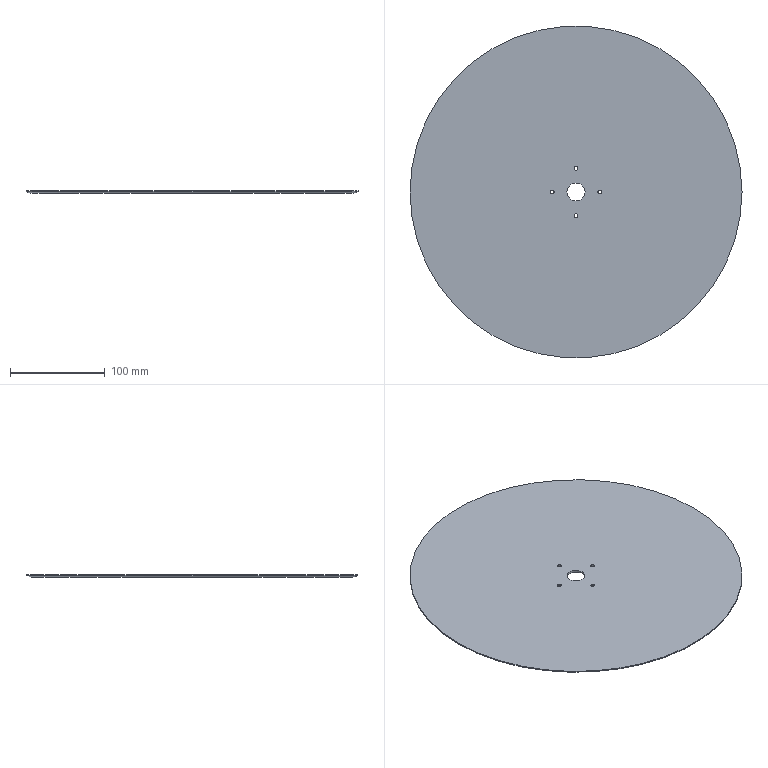Part | SolidWorks | features ICE 3, Extrusion 1, Sweep 1 | 1 solid | 16 faces | box 350 x 350 x 2.3 mm | volume 217251 mm3 | cylinder 12 | cone 2 | plane 2 | commonest cylinder face diameters 4 x8 19 x2 350 x2
STEP:
#1=CARTESIAN_POINT('',(-27.,0.,-1.2));
#2=VERTEX_POINT('',#1);
#3=CARTESIAN_POINT('',(-23.,0.,-1.2));
#4=VERTEX_POINT('',#3);
#5=CARTESIAN_POINT('',(-25.,0.,-1.2));
#6=DIRECTION('',(0.,0.,1.));
#7=DIRECTION('',(-1.,0.,0.));
#8=AXIS2_PLACEMENT_3D('',#5,#6,#7);
#9=CIRCLE('',#8,2.);
#10=EDGE_CURVE('',#2,#4,#9,.T.);
#11=ORIENTED_EDGE('',*,*,#10,.F.);
#12=CARTESIAN_POINT('',(-27.,0.,1.1));
#13=VERTEX_POINT('',#12);
#14=CARTESIAN_POINT('',(-27.,0.,-6.857));
#15=DIRECTION('',(0.,0.,1.));
#16=VECTOR('',#15,1000.);
#17=LINE('',#14,#16);
#18=EDGE_CURVE('',#2,#13,#17,.T.);
#19=ORIENTED_EDGE('',*,*,#18,.T.);
#20=CARTESIAN_POINT('',(-23.,0.,1.1));
#21=VERTEX_POINT('',#20);
#22=CARTESIAN_POINT('',(-25.,0.,1.1));
#23=DIRECTION('',(0.,0.,1.));
#24=DIRECTION('',(1.,0.,0.));
#25=AXIS2_PLACEMENT_3D('',#22,#23,#24);
#26=CIRCLE('',#25,2.);
#27=EDGE_CURVE('',#13,#21,#26,.T.);
#28=ORIENTED_EDGE('',*,*,#27,.T.);
#29=CARTESIAN_POINT('',(-23.,0.,-6.857));
#30=DIRECTION('',(0.,0.,1.));
#31=VECTOR('',#30,1000.);
#32=LINE('',#29,#31);
#33=EDGE_CURVE('',#4,#21,#32,.T.);
#34=ORIENTED_EDGE('',*,*,#33,.F.);
#35=EDGE_LOOP('',(#11,#19,#28,#34));
#36=FACE_OUTER_BOUND('',#35,.T.);
#37=CARTESIAN_POINT('',(-25.,0.,-6.857));
#38=DIRECTION('',(0.,0.,1.));
#39=DIRECTION('',(1.,0.,0.));
#40=AXIS2_PLACEMENT_3D('',#37,#38,#39);
#41=CYLINDRICAL_SURFACE('',#40,2.);
#42=ADVANCED_FACE('',(#36),#41,.F.);
#43=CARTESIAN_POINT('',(-2.,-25.,-1.2));
#44=VERTEX_POINT('',#43);
#45=CARTESIAN_POINT('',(2.,-25.,-1.2));
#46=VERTEX_POINT('',#45);
#47=CARTESIAN_POINT('',(0.,-25.,-1.2));
#48=DIRECTION('',(0.,0.,1.));
#49=DIRECTION('',(-1.,0.,0.));
#50=AXIS2_PLACEMENT_3D('',#47,#48,#49);
#51=CIRCLE('',#50,2.);
#52=EDGE_CURVE('',#44,#46,#51,.T.);
#53=ORIENTED_EDGE('',*,*,#52,.F.);
#54=CARTESIAN_POINT('',(-2.,-25.,1.1));
#55=VERTEX_POINT('',#54);
#56=CARTESIAN_POINT('',(-2.,-25.,-6.857));
#57=DIRECTION('',(0.,0.,1.));
#58=VECTOR('',#57,1000.);
#59=LINE('',#56,#58);
#60=EDGE_CURVE('',#44,#55,#59,.T.);
#61=ORIENTED_EDGE('',*,*,#60,.T.);
#62=CARTESIAN_POINT('',(2.,-25.,1.1));
#63=VERTEX_POINT('',#62);
#64=CARTESIAN_POINT('',(0.,-25.,1.1));
#65=DIRECTION('',(0.,0.,1.));
#66=DIRECTION('',(1.,0.,0.));
#67=AXIS2_PLACEMENT_3D('',#64,#65,#66);
#68=CIRCLE('',#67,2.);
#69=EDGE_CURVE('',#55,#63,#68,.T.);
#70=ORIENTED_EDGE('',*,*,#69,.T.);
#71=CARTESIAN_POINT('',(2.,-25.,-6.857));
#72=DIRECTION('',(0.,0.,1.));
#73=VECTOR('',#72,1000.);
#74=LINE('',#71,#73);
#75=EDGE_CURVE('',#46,#63,#74,.T.);
#76=ORIENTED_EDGE('',*,*,#75,.F.);
#77=EDGE_LOOP('',(#53,#61,#70,#76));
#78=FACE_OUTER_BOUND('',#77,.T.);
#79=CARTESIAN_POINT('',(0.,-25.,-6.857));
#80=DIRECTION('',(0.,0.,1.));
#81=DIRECTION('',(1.,0.,0.));
#82=AXIS2_PLACEMENT_3D('',#79,#80,#81);
#83=CYLINDRICAL_SURFACE('',#82,2.);
#84=ADVANCED_FACE('',(#78),#83,.F.);
#85=CARTESIAN_POINT('',(23.,0.,-1.2));
#86=VERTEX_POINT('',#85);
#87=CARTESIAN_POINT('',(27.,0.,-1.2));
#88=VERTEX_POINT('',#87);
#89=CARTESIAN_POINT('',(25.,0.,-1.2));
#90=DIRECTION('',(0.,0.,1.));
#91=DIRECTION('',(-1.,0.,0.));
#92=AXIS2_PLACEMENT_3D('',#89,#90,#91);
#93=CIRCLE('',#92,2.);
#94=EDGE_CURVE('',#86,#88,#93,.T.);
#95=ORIENTED_EDGE('',*,*,#94,.F.);
#96=CARTESIAN_POINT('',(23.,0.,1.1));
#97=VERTEX_POINT('',#96);
#98=CARTESIAN_POINT('',(23.,0.,-6.857));
#99=DIRECTION('',(0.,0.,1.));
#100=VECTOR('',#99,1000.);
#101=LINE('',#98,#100);
#102=EDGE_CURVE('',#86,#97,#101,.T.);
#103=ORIENTED_EDGE('',*,*,#102,.T.);
#104=CARTESIAN_POINT('',(27.,0.,1.1));
#105=VERTEX_POINT('',#104);
#106=CARTESIAN_POINT('',(25.,0.,1.1));
#107=DIRECTION('',(0.,0.,1.));
#108=DIRECTION('',(1.,0.,0.));
#109=AXIS2_PLACEMENT_3D('',#106,#107,#108);
#110=CIRCLE('',#109,2.);
#111=EDGE_CURVE('',#97,#105,#110,.T.);
#112=ORIENTED_EDGE('',*,*,#111,.T.);
#113=CARTESIAN_POINT('',(27.,0.,-6.857));
#114=DIRECTION('',(0.,0.,1.));
#115=VECTOR('',#114,1000.);
#116=LINE('',#113,#115);
#117=EDGE_CURVE('',#88,#105,#116,.T.);
#118=ORIENTED_EDGE('',*,*,#117,.F.);
#119=EDGE_LOOP('',(#95,#103,#112,#118));
#120=FACE_OUTER_BOUND('',#119,.T.);
#121=CARTESIAN_POINT('',(25.,0.,-6.857));
#122=DIRECTION('',(0.,0.,1.));
#123=DIRECTION('',(1.,0.,0.));
#124=AXIS2_PLACEMENT_3D('',#121,#122,#123);
#125=CYLINDRICAL_SURFACE('',#124,2.);
#126=ADVANCED_FACE('',(#120),#125,.F.);
#127=CARTESIAN_POINT('',(-2.,25.,-1.2));
#128=VERTEX_POINT('',#127);
#129=CARTESIAN_POINT('',(2.,25.,-1.2));
#130=VERTEX_POINT('',#129);
#131=CARTESIAN_POINT('',(0.,25.,-1.2));
#132=DIRECTION('',(0.,0.,1.));
#133=DIRECTION('',(-1.,0.,0.));
#134=AXIS2_PLACEMENT_3D('',#131,#132,#133);
#135=CIRCLE('',#134,2.);
#136=EDGE_CURVE('',#128,#130,#135,.T.);
#137=ORIENTED_EDGE('',*,*,#136,.F.);
#138=CARTESIAN_POINT('',(-2.,25.,1.1));
#139=VERTEX_POINT('',#138);
#140=CARTESIAN_POINT('',(-2.,25.,-6.857));
#141=DIRECTION('',(0.,0.,1.));
#142=VECTOR('',#141,1000.);
#143=LINE('',#140,#142);
#144=EDGE_CURVE('',#128,#139,#143,.T.);
#145=ORIENTED_EDGE('',*,*,#144,.T.);
#146=CARTESIAN_POINT('',(2.,25.,1.1));
#147=VERTEX_POINT('',#146);
#148=CARTESIAN_POINT('',(0.,25.,1.1));
#149=DIRECTION('',(0.,0.,1.));
#150=DIRECTION('',(1.,0.,0.));
#151=AXIS2_PLACEMENT_3D('',#148,#149,#150);
#152=CIRCLE('',#151,2.);
#153=EDGE_CURVE('',#139,#147,#152,.T.);
#154=ORIENTED_EDGE('',*,*,#153,.T.);
#155=CARTESIAN_POINT('',(2.,25.,-6.857));
#156=DIRECTION('',(0.,0.,1.));
#157=VECTOR('',#156,1000.);
#158=LINE('',#155,#157);
#159=EDGE_CURVE('',#130,#147,#158,.T.);
#160=ORIENTED_EDGE('',*,*,#159,.F.);
#161=EDGE_LOOP('',(#137,#145,#154,#160));
#162=FACE_OUTER_BOUND('',#161,.T.);
#163=CARTESIAN_POINT('',(0.,25.,-6.857));
#164=DIRECTION('',(0.,0.,1.));
#165=DIRECTION('',(1.,0.,0.));
#166=AXIS2_PLACEMENT_3D('',#163,#164,#165);
#167=CYLINDRICAL_SURFACE('',#166,2.);
#168=ADVANCED_FACE('',(#162),#167,.F.);
#169=CARTESIAN_POINT('',(170.,0.,-1.2));
#170=VERTEX_POINT('',#169);
#171=CARTESIAN_POINT('',(-170.,0.,-1.2));
#172=VERTEX_POINT('',#171);
#173=CARTESIAN_POINT('',(0.,0.,-1.2));
#174=DIRECTION('',(0.,0.,1.));
#175=DIRECTION('',(1.,0.,0.));
#176=AXIS2_PLACEMENT_3D('',#173,#174,#175);
#177=CIRCLE('',#176,170.);
#178=EDGE_CURVE('',#170,#172,#177,.T.);
#179=ORIENTED_EDGE('',*,*,#178,.T.);
#180=CARTESIAN_POINT('',(-175.,0.,0.));
#181=VERTEX_POINT('',#180);
#182=CARTESIAN_POINT('',(-170.,0.,-1.2));
#183=DIRECTION('',(-0.9724,0.,0.2334));
#184=VECTOR('',#183,1000.);
#185=LINE('',#182,#184);
#186=EDGE_CURVE('',#172,#181,#185,.T.);
#187=ORIENTED_EDGE('',*,*,#186,.T.);
#188=CARTESIAN_POINT('',(175.,0.,0.));
#189=VERTEX_POINT('',#188);
#190=CARTESIAN_POINT('',(0.,0.,0.));
#191=DIRECTION('',(0.,0.,1.));
#192=DIRECTION('',(1.,0.,0.));
#193=AXIS2_PLACEMENT_3D('',#190,#191,#192);
#194=CIRCLE('',#193,175.);
#195=EDGE_CURVE('',#189,#181,#194,.T.);
#196=ORIENTED_EDGE('',*,*,#195,.F.);
#197=CARTESIAN_POINT('',(170.,0.,-1.2));
#198=DIRECTION('',(0.9724,0.,0.2334));
#199=VECTOR('',#198,1000.);
#200=LINE('',#197,#199);
#201=EDGE_CURVE('',#170,#189,#200,.T.);
#202=ORIENTED_EDGE('',*,*,#201,.F.);
#203=EDGE_LOOP('',(#179,#187,#196,#202));
#204=FACE_OUTER_BOUND('',#203,.T.);
#205=CARTESIAN_POINT('',(0.,0.,-1.2));
#206=DIRECTION('',(0.,0.,1.));
#207=DIRECTION('',(1.,0.,0.));
#208=AXIS2_PLACEMENT_3D('',#205,#206,#207);
#209=CONICAL_SURFACE('',#208,170.,1.335);
#210=ADVANCED_FACE('',(#204),#209,.T.);
#211=CARTESIAN_POINT('',(-9.5,0.,-1.2));
#212=VERTEX_POINT('',#211);
#213=CARTESIAN_POINT('',(9.5,0.,-1.2));
#214=VERTEX_POINT('',#213);
#215=CARTESIAN_POINT('',(0.,0.,-1.2));
#216=DIRECTION('',(0.,0.,1.));
#217=DIRECTION('',(1.,0.,0.));
#218=AXIS2_PLACEMENT_3D('',#215,#216,#217);
#219=CIRCLE('',#218,9.5);
#220=EDGE_CURVE('',#212,#214,#219,.T.);
#221=ORIENTED_EDGE('',*,*,#220,.F.);
#222=CARTESIAN_POINT('',(-9.5,0.,1.1));
#223=VERTEX_POINT('',#222);
#224=CARTESIAN_POINT('',(-9.5,0.,-1.2));
#225=DIRECTION('',(0.,0.,1.));
#226=VECTOR('',#225,1000.);
#227=LINE('',#224,#226);
#228=EDGE_CURVE('',#212,#223,#227,.T.);
#229=ORIENTED_EDGE('',*,*,#228,.T.);
#230=CARTESIAN_POINT('',(9.5,0.,1.1));
#231=VERTEX_POINT('',#230);
#232=CARTESIAN_POINT('',(0.,0.,1.1));
#233=DIRECTION('',(0.,0.,1.));
#234=DIRECTION('',(1.,0.,0.));
#235=AXIS2_PLACEMENT_3D('',#232,#233,#234);
#236=CIRCLE('',#235,9.5);
#237=EDGE_CURVE('',#223,#231,#236,.T.);
#238=ORIENTED_EDGE('',*,*,#237,.T.);
#239=CARTESIAN_POINT('',(9.5,0.,-1.2));
#240=DIRECTION('',(0.,0.,1.));
#241=VECTOR('',#240,1000.);
#242=LINE('',#239,#241);
#243=EDGE_CURVE('',#214,#231,#242,.T.);
#244=ORIENTED_EDGE('',*,*,#243,.F.);
#245=EDGE_LOOP('',(#221,#229,#238,#244));
#246=FACE_OUTER_BOUND('',#245,.T.);
#247=CARTESIAN_POINT('',(0.,0.,-1.2));
#248=DIRECTION('',(0.,0.,1.));
#249=DIRECTION('',(1.,0.,0.));
#250=AXIS2_PLACEMENT_3D('',#247,#248,#249);
#251=CYLINDRICAL_SURFACE('',#250,9.5);
#252=ADVANCED_FACE('',(#246),#251,.F.);
#253=CARTESIAN_POINT('',(175.,0.,1.1));
#254=VERTEX_POINT('',#253);
#255=CARTESIAN_POINT('',(-175.,0.,1.1));
#256=VERTEX_POINT('',#255);
#257=CARTESIAN_POINT('',(0.,0.,1.1));
#258=DIRECTION('',(0.,0.,1.));
#259=DIRECTION('',(1.,0.,0.));
#260=AXIS2_PLACEMENT_3D('',#257,#258,#259);
#261=CIRCLE('',#260,175.);
#262=EDGE_CURVE('',#254,#256,#261,.T.);
#263=ORIENTED_EDGE('',*,*,#262,.F.);
#264=CARTESIAN_POINT('',(175.,0.,1.1));
#265=DIRECTION('',(0.,0.,-1.));
#266=VECTOR('',#265,1000.);
#267=LINE('',#264,#266);
#268=EDGE_CURVE('',#254,#189,#267,.T.);
#269=ORIENTED_EDGE('',*,*,#268,.T.);
#270=ORIENTED_EDGE('',*,*,#195,.T.);
#271=CARTESIAN_POINT('',(-175.,0.,1.1));
#272=DIRECTION('',(0.,0.,-1.));
#273=VECTOR('',#272,1000.);
#274=LINE('',#271,#273);
#275=EDGE_CURVE('',#256,#181,#274,.T.);
#276=ORIENTED_EDGE('',*,*,#275,.F.);
#277=EDGE_LOOP('',(#263,#269,#270,#276));
#278=FACE_OUTER_BOUND('',#277,.T.);
#279=CARTESIAN_POINT('',(0.,0.,1.1));
#280=DIRECTION('',(0.,0.,-1.));
#281=DIRECTION('',(-1.,0.,0.));
#282=AXIS2_PLACEMENT_3D('',#279,#280,#281);
#283=CYLINDRICAL_SURFACE('',#282,175.);
#284=ADVANCED_FACE('',(#278),#283,.T.);
#285=ORIENTED_EDGE('',*,*,#268,.F.);
#286=CARTESIAN_POINT('',(0.,0.,1.1));
#287=DIRECTION('',(0.,0.,1.));
#288=DIRECTION('',(1.,0.,0.));
#289=AXIS2_PLACEMENT_3D('',#286,#287,#288);
#290=CIRCLE('',#289,175.);
#291=EDGE_CURVE('',#256,#254,#290,.T.);
#292=ORIENTED_EDGE('',*,*,#291,.F.);
#293=ORIENTED_EDGE('',*,*,#275,.T.);
#294=CARTESIAN_POINT('',(0.,0.,0.));
#295=DIRECTION('',(0.,0.,1.));
#296=DIRECTION('',(1.,0.,0.));
#297=AXIS2_PLACEMENT_3D('',#294,#295,#296);
#298=CIRCLE('',#297,175.);
#299=EDGE_CURVE('',#181,#189,#298,.T.);
#300=ORIENTED_EDGE('',*,*,#299,.T.);
#301=EDGE_LOOP('',(#285,#292,#293,#300));
#302=FACE_OUTER_BOUND('',#301,.T.);
#303=CARTESIAN_POINT('',(0.,0.,1.1));
#304=DIRECTION('',(0.,0.,-1.));
#305=DIRECTION('',(-1.,0.,0.));
#306=AXIS2_PLACEMENT_3D('',#303,#304,#305);
#307=CYLINDRICAL_SURFACE('',#306,175.);
#308=ADVANCED_FACE('',(#302),#307,.T.);
#309=CARTESIAN_POINT('',(-25.,0.,1.1));
#310=DIRECTION('',(0.,0.,1.));
#311=DIRECTION('',(1.,0.,0.));
#312=AXIS2_PLACEMENT_3D('',#309,#310,#311);
#313=CIRCLE('',#312,2.);
#314=EDGE_CURVE('',#21,#13,#313,.T.);
#315=ORIENTED_EDGE('',*,*,#314,.F.);
#316=ORIENTED_EDGE('',*,*,#27,.F.);
#317=EDGE_LOOP('',(#315,#316));
#318=FACE_BOUND('',#317,.T.);
#319=CARTESIAN_POINT('',(0.,-25.,1.1));
#320=DIRECTION('',(0.,0.,1.));
#321=DIRECTION('',(1.,0.,0.));
#322=AXIS2_PLACEMENT_3D('',#319,#320,#321);
#323=CIRCLE('',#322,2.);
#324=EDGE_CURVE('',#63,#55,#323,.T.);
#325=ORIENTED_EDGE('',*,*,#324,.F.);
#326=ORIENTED_EDGE('',*,*,#69,.F.);
#327=EDGE_LOOP('',(#325,#326));
#328=FACE_BOUND('',#327,.T.);
#329=CARTESIAN_POINT('',(25.,0.,1.1));
#330=DIRECTION('',(0.,0.,1.));
#331=DIRECTION('',(1.,0.,0.));
#332=AXIS2_PLACEMENT_3D('',#329,#330,#331);
#333=CIRCLE('',#332,2.);
#334=EDGE_CURVE('',#105,#97,#333,.T.);
#335=ORIENTED_EDGE('',*,*,#334,.F.);
#336=ORIENTED_EDGE('',*,*,#111,.F.);
#337=EDGE_LOOP('',(#335,#336));
#338=FACE_BOUND('',#337,.T.);
#339=CARTESIAN_POINT('',(0.,25.,1.1));
#340=DIRECTION('',(0.,0.,1.));
#341=DIRECTION('',(1.,0.,0.));
#342=AXIS2_PLACEMENT_3D('',#339,#340,#341);
#343=CIRCLE('',#342,2.);
#344=EDGE_CURVE('',#147,#139,#343,.T.);
#345=ORIENTED_EDGE('',*,*,#344,.F.);
#346=ORIENTED_EDGE('',*,*,#153,.F.);
#347=EDGE_LOOP('',(#345,#346));
#348=FACE_BOUND('',#347,.T.);
#349=CARTESIAN_POINT('',(0.,0.,1.1));
#350=DIRECTION('',(0.,0.,1.));
#351=DIRECTION('',(1.,0.,0.));
#352=AXIS2_PLACEMENT_3D('',#349,#350,#351);
#353=CIRCLE('',#352,9.5);
#354=EDGE_CURVE('',#231,#223,#353,.T.);
#355=ORIENTED_EDGE('',*,*,#354,.F.);
#356=ORIENTED_EDGE('',*,*,#237,.F.);
#357=EDGE_LOOP('',(#355,#356));
#358=FACE_BOUND('',#357,.T.);
#359=ORIENTED_EDGE('',*,*,#291,.T.);
#360=ORIENTED_EDGE('',*,*,#262,.T.);
#361=EDGE_LOOP('',(#359,#360));
#362=FACE_OUTER_BOUND('',#361,.T.);
#363=CARTESIAN_POINT('',(0.,0.,1.1));
#364=DIRECTION('',(0.,0.,1.));
#365=DIRECTION('',(1.,0.,0.));
#366=AXIS2_PLACEMENT_3D('',#363,#364,#365);
#367=PLANE('',#366);
#368=ADVANCED_FACE('',(#318,#328,#338,#348,#358,#362),#367,.T.);
#369=CARTESIAN_POINT('',(-25.,0.,-1.2));
#370=DIRECTION('',(0.,0.,1.));
#371=DIRECTION('',(-1.,0.,0.));
#372=AXIS2_PLACEMENT_3D('',#369,#370,#371);
#373=CIRCLE('',#372,2.);
#374=EDGE_CURVE('',#4,#2,#373,.T.);
#375=ORIENTED_EDGE('',*,*,#374,.T.);
#376=ORIENTED_EDGE('',*,*,#10,.T.);
#377=EDGE_LOOP('',(#375,#376));
#378=FACE_BOUND('',#377,.T.);
#379=CARTESIAN_POINT('',(0.,-25.,-1.2));
#380=DIRECTION('',(0.,0.,1.));
#381=DIRECTION('',(-1.,0.,0.));
#382=AXIS2_PLACEMENT_3D('',#379,#380,#381);
#383=CIRCLE('',#382,2.);
#384=EDGE_CURVE('',#46,#44,#383,.T.);
#385=ORIENTED_EDGE('',*,*,#384,.T.);
#386=ORIENTED_EDGE('',*,*,#52,.T.);
#387=EDGE_LOOP('',(#385,#386));
#388=FACE_BOUND('',#387,.T.);
#389=CARTESIAN_POINT('',(25.,0.,-1.2));
#390=DIRECTION('',(0.,0.,1.));
#391=DIRECTION('',(-1.,0.,0.));
#392=AXIS2_PLACEMENT_3D('',#389,#390,#391);
#393=CIRCLE('',#392,2.);
#394=EDGE_CURVE('',#88,#86,#393,.T.);
#395=ORIENTED_EDGE('',*,*,#394,.T.);
#396=ORIENTED_EDGE('',*,*,#94,.T.);
#397=EDGE_LOOP('',(#395,#396));
#398=FACE_BOUND('',#397,.T.);
#399=CARTESIAN_POINT('',(0.,25.,-1.2));
#400=DIRECTION('',(0.,0.,1.));
#401=DIRECTION('',(-1.,0.,0.));
#402=AXIS2_PLACEMENT_3D('',#399,#400,#401);
#403=CIRCLE('',#402,2.);
#404=EDGE_CURVE('',#130,#128,#403,.T.);
#405=ORIENTED_EDGE('',*,*,#404,.T.);
#406=ORIENTED_EDGE('',*,*,#136,.T.);
#407=EDGE_LOOP('',(#405,#406));
#408=FACE_BOUND('',#407,.T.);
#409=CARTESIAN_POINT('',(0.,0.,-1.2));
#410=DIRECTION('',(0.,0.,1.));
#411=DIRECTION('',(1.,0.,0.));
#412=AXIS2_PLACEMENT_3D('',#409,#410,#411);
#413=CIRCLE('',#412,9.5);
#414=EDGE_CURVE('',#214,#212,#413,.T.);
#415=ORIENTED_EDGE('',*,*,#414,.T.);
#416=ORIENTED_EDGE('',*,*,#220,.T.);
#417=EDGE_LOOP('',(#415,#416));
#418=FACE_BOUND('',#417,.T.);
#419=ORIENTED_EDGE('',*,*,#178,.F.);
#420=CARTESIAN_POINT('',(0.,0.,-1.2));
#421=DIRECTION('',(0.,0.,1.));
#422=DIRECTION('',(1.,0.,0.));
#423=AXIS2_PLACEMENT_3D('',#420,#421,#422);
#424=CIRCLE('',#423,170.);
#425=EDGE_CURVE('',#172,#170,#424,.T.);
#426=ORIENTED_EDGE('',*,*,#425,.F.);
#427=EDGE_LOOP('',(#419,#426));
#428=FACE_OUTER_BOUND('',#427,.T.);
#429=CARTESIAN_POINT('',(0.,0.,-1.2));
#430=DIRECTION('',(0.,0.,-1.));
#431=DIRECTION('',(-1.,0.,0.));
#432=AXIS2_PLACEMENT_3D('',#429,#430,#431);
#433=PLANE('',#432);
#434=ADVANCED_FACE('',(#378,#388,#398,#408,#418,#428),#433,.T.);
#435=ORIENTED_EDGE('',*,*,#228,.F.);
#436=ORIENTED_EDGE('',*,*,#414,.F.);
#437=ORIENTED_EDGE('',*,*,#243,.T.);
#438=ORIENTED_EDGE('',*,*,#354,.T.);
#439=EDGE_LOOP('',(#435,#436,#437,#438));
#440=FACE_OUTER_BOUND('',#439,.T.);
#441=CARTESIAN_POINT('',(0.,0.,-1.2));
#442=DIRECTION('',(0.,0.,1.));
#443=DIRECTION('',(1.,0.,0.));
#444=AXIS2_PLACEMENT_3D('',#441,#442,#443);
#445=CYLINDRICAL_SURFACE('',#444,9.5);
#446=ADVANCED_FACE('',(#440),#445,.F.);
#447=ORIENTED_EDGE('',*,*,#186,.F.);
#448=ORIENTED_EDGE('',*,*,#425,.T.);
#449=ORIENTED_EDGE('',*,*,#201,.T.);
#450=ORIENTED_EDGE('',*,*,#299,.F.);
#451=EDGE_LOOP('',(#447,#448,#449,#450));
#452=FACE_OUTER_BOUND('',#451,.T.);
#453=CARTESIAN_POINT('',(0.,0.,-1.2));
#454=DIRECTION('',(0.,0.,1.));
#455=DIRECTION('',(1.,0.,0.));
#456=AXIS2_PLACEMENT_3D('',#453,#454,#455);
#457=CONICAL_SURFACE('',#456,170.,1.335);
#458=ADVANCED_FACE('',(#452),#457,.T.);
#459=ORIENTED_EDGE('',*,*,#144,.F.);
#460=ORIENTED_EDGE('',*,*,#404,.F.);
#461=ORIENTED_EDGE('',*,*,#159,.T.);
#462=ORIENTED_EDGE('',*,*,#344,.T.);
#463=EDGE_LOOP('',(#459,#460,#461,#462));
#464=FACE_OUTER_BOUND('',#463,.T.);
#465=CARTESIAN_POINT('',(0.,25.,-6.857));
#466=DIRECTION('',(0.,0.,1.));
#467=DIRECTION('',(1.,0.,0.));
#468=AXIS2_PLACEMENT_3D('',#465,#466,#467);
#469=CYLINDRICAL_SURFACE('',#468,2.);
#470=ADVANCED_FACE('',(#464),#469,.F.);
#471=ORIENTED_EDGE('',*,*,#102,.F.);
#472=ORIENTED_EDGE('',*,*,#394,.F.);
#473=ORIENTED_EDGE('',*,*,#117,.T.);
#474=ORIENTED_EDGE('',*,*,#334,.T.);
#475=EDGE_LOOP('',(#471,#472,#473,#474));
#476=FACE_OUTER_BOUND('',#475,.T.);
#477=CARTESIAN_POINT('',(25.,0.,-6.857));
#478=DIRECTION('',(0.,0.,1.));
#479=DIRECTION('',(1.,0.,0.));
#480=AXIS2_PLACEMENT_3D('',#477,#478,#479);
#481=CYLINDRICAL_SURFACE('',#480,2.);
#482=ADVANCED_FACE('',(#476),#481,.F.);
#483=ORIENTED_EDGE('',*,*,#60,.F.);
#484=ORIENTED_EDGE('',*,*,#384,.F.);
#485=ORIENTED_EDGE('',*,*,#75,.T.);
#486=ORIENTED_EDGE('',*,*,#324,.T.);
#487=EDGE_LOOP('',(#483,#484,#485,#486));
#488=FACE_OUTER_BOUND('',#487,.T.);
#489=CARTESIAN_POINT('',(0.,-25.,-6.857));
#490=DIRECTION('',(0.,0.,1.));
#491=DIRECTION('',(1.,0.,0.));
#492=AXIS2_PLACEMENT_3D('',#489,#490,#491);
#493=CYLINDRICAL_SURFACE('',#492,2.);
#494=ADVANCED_FACE('',(#488),#493,.F.);
#495=ORIENTED_EDGE('',*,*,#18,.F.);
#496=ORIENTED_EDGE('',*,*,#374,.F.);
#497=ORIENTED_EDGE('',*,*,#33,.T.);
#498=ORIENTED_EDGE('',*,*,#314,.T.);
#499=EDGE_LOOP('',(#495,#496,#497,#498));
#500=FACE_OUTER_BOUND('',#499,.T.);
#501=CARTESIAN_POINT('',(-25.,0.,-6.857));
#502=DIRECTION('',(0.,0.,1.));
#503=DIRECTION('',(1.,0.,0.));
#504=AXIS2_PLACEMENT_3D('',#501,#502,#503);
#505=CYLINDRICAL_SURFACE('',#504,2.);
#506=ADVANCED_FACE('',(#500),#505,.F.);
#507=CLOSED_SHELL('',(#42,#84,#126,#168,#210,#252,#284,#308,#368,#434,#446,#458,#470,#482,#494,#506));
#508=MANIFOLD_SOLID_BREP('',#507);
#509=CARTESIAN_POINT('',(0.,0.,0.));
#510=DIRECTION('',(0.,0.,1.));
#511=DIRECTION('',(1.,0.,0.));
#512=AXIS2_PLACEMENT_3D('',#509,#510,#511);
#513=(LENGTH_UNIT()NAMED_UNIT(*)SI_UNIT(.MILLI.,.METRE.));
#514=UNCERTAINTY_MEASURE_WITH_UNIT(LENGTH_MEASURE(0.00001),#513,'','');
#515=(NAMED_UNIT(*)PLANE_ANGLE_UNIT()SI_UNIT($,.RADIAN.));
#516=(NAMED_UNIT(*)SI_UNIT($,.STERADIAN.)SOLID_ANGLE_UNIT());
#517=(GEOMETRIC_REPRESENTATION_CONTEXT(3)GLOBAL_UNCERTAINTY_ASSIGNED_CONTEXT((#514))GLOBAL_UNIT_ASSIGNED_CONTEXT((#513,#515,#516))REPRESENTATION_CONTEXT('',''));
#518=ADVANCED_BREP_SHAPE_REPRESENTATION('',(#508,#512),#517);